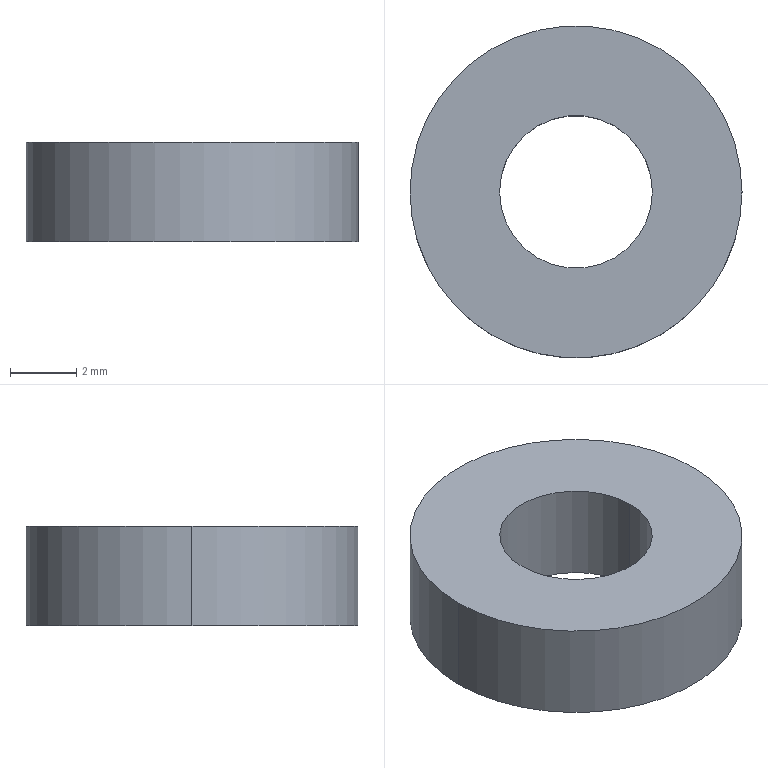Part | SolidWorks | features Extrusion 1 | 1 solid | 6 faces | box 10 x 10 x 3 mm | volume 185.762 mm3 | cylinder 4 | plane 2 | commonest cylinder face diameters 4.6 x2 10 x2
STEP:
#1=CARTESIAN_POINT('',(-2.3,0.,3.));
#2=VERTEX_POINT('',#1);
#3=CARTESIAN_POINT('',(2.3,0.,3.));
#4=VERTEX_POINT('',#3);
#5=CARTESIAN_POINT('',(0.,0.,3.));
#6=DIRECTION('',(0.,0.,1.));
#7=DIRECTION('',(1.,0.,0.));
#8=AXIS2_PLACEMENT_3D('',#5,#6,#7);
#9=CIRCLE('',#8,2.3);
#10=EDGE_CURVE('',#2,#4,#9,.T.);
#11=ORIENTED_EDGE('',*,*,#10,.T.);
#12=CARTESIAN_POINT('',(2.3,0.,0.));
#13=VERTEX_POINT('',#12);
#14=CARTESIAN_POINT('',(2.3,0.,3.));
#15=DIRECTION('',(0.,0.,-1.));
#16=VECTOR('',#15,1000.);
#17=LINE('',#14,#16);
#18=EDGE_CURVE('',#4,#13,#17,.T.);
#19=ORIENTED_EDGE('',*,*,#18,.T.);
#20=CARTESIAN_POINT('',(-2.3,0.,0.));
#21=VERTEX_POINT('',#20);
#22=CARTESIAN_POINT('',(0.,0.,0.));
#23=DIRECTION('',(0.,0.,1.));
#24=DIRECTION('',(1.,0.,0.));
#25=AXIS2_PLACEMENT_3D('',#22,#23,#24);
#26=CIRCLE('',#25,2.3);
#27=EDGE_CURVE('',#21,#13,#26,.T.);
#28=ORIENTED_EDGE('',*,*,#27,.F.);
#29=CARTESIAN_POINT('',(-2.3,0.,3.));
#30=DIRECTION('',(0.,0.,-1.));
#31=VECTOR('',#30,1000.);
#32=LINE('',#29,#31);
#33=EDGE_CURVE('',#2,#21,#32,.T.);
#34=ORIENTED_EDGE('',*,*,#33,.F.);
#35=EDGE_LOOP('',(#11,#19,#28,#34));
#36=FACE_OUTER_BOUND('',#35,.T.);
#37=CARTESIAN_POINT('',(0.,0.,3.));
#38=DIRECTION('',(0.,0.,-1.));
#39=DIRECTION('',(-1.,0.,0.));
#40=AXIS2_PLACEMENT_3D('',#37,#38,#39);
#41=CYLINDRICAL_SURFACE('',#40,2.3);
#42=ADVANCED_FACE('',(#36),#41,.F.);
#43=CARTESIAN_POINT('',(5.,0.,3.));
#44=VERTEX_POINT('',#43);
#45=CARTESIAN_POINT('',(-5.,0.,3.));
#46=VERTEX_POINT('',#45);
#47=CARTESIAN_POINT('',(0.,0.,3.));
#48=DIRECTION('',(0.,0.,1.));
#49=DIRECTION('',(1.,0.,0.));
#50=AXIS2_PLACEMENT_3D('',#47,#48,#49);
#51=CIRCLE('',#50,5.);
#52=EDGE_CURVE('',#44,#46,#51,.T.);
#53=ORIENTED_EDGE('',*,*,#52,.F.);
#54=CARTESIAN_POINT('',(5.,0.,0.));
#55=VERTEX_POINT('',#54);
#56=CARTESIAN_POINT('',(5.,0.,3.));
#57=DIRECTION('',(0.,0.,-1.));
#58=VECTOR('',#57,1000.);
#59=LINE('',#56,#58);
#60=EDGE_CURVE('',#44,#55,#59,.T.);
#61=ORIENTED_EDGE('',*,*,#60,.T.);
#62=CARTESIAN_POINT('',(-5.,0.,0.));
#63=VERTEX_POINT('',#62);
#64=CARTESIAN_POINT('',(0.,0.,0.));
#65=DIRECTION('',(0.,0.,1.));
#66=DIRECTION('',(1.,0.,0.));
#67=AXIS2_PLACEMENT_3D('',#64,#65,#66);
#68=CIRCLE('',#67,5.);
#69=EDGE_CURVE('',#55,#63,#68,.T.);
#70=ORIENTED_EDGE('',*,*,#69,.T.);
#71=CARTESIAN_POINT('',(-5.,0.,3.));
#72=DIRECTION('',(0.,0.,-1.));
#73=VECTOR('',#72,1000.);
#74=LINE('',#71,#73);
#75=EDGE_CURVE('',#46,#63,#74,.T.);
#76=ORIENTED_EDGE('',*,*,#75,.F.);
#77=EDGE_LOOP('',(#53,#61,#70,#76));
#78=FACE_OUTER_BOUND('',#77,.T.);
#79=CARTESIAN_POINT('',(0.,0.,3.));
#80=DIRECTION('',(0.,0.,-1.));
#81=DIRECTION('',(-1.,0.,0.));
#82=AXIS2_PLACEMENT_3D('',#79,#80,#81);
#83=CYLINDRICAL_SURFACE('',#82,5.);
#84=ADVANCED_FACE('',(#78),#83,.T.);
#85=CARTESIAN_POINT('',(0.,0.,3.));
#86=DIRECTION('',(0.,0.,1.));
#87=DIRECTION('',(1.,0.,0.));
#88=AXIS2_PLACEMENT_3D('',#85,#86,#87);
#89=CIRCLE('',#88,5.);
#90=EDGE_CURVE('',#46,#44,#89,.T.);
#91=ORIENTED_EDGE('',*,*,#90,.T.);
#92=ORIENTED_EDGE('',*,*,#52,.T.);
#93=EDGE_LOOP('',(#91,#92));
#94=FACE_OUTER_BOUND('',#93,.T.);
#95=ORIENTED_EDGE('',*,*,#10,.F.);
#96=CARTESIAN_POINT('',(0.,0.,3.));
#97=DIRECTION('',(0.,0.,1.));
#98=DIRECTION('',(1.,0.,0.));
#99=AXIS2_PLACEMENT_3D('',#96,#97,#98);
#100=CIRCLE('',#99,2.3);
#101=EDGE_CURVE('',#4,#2,#100,.T.);
#102=ORIENTED_EDGE('',*,*,#101,.F.);
#103=EDGE_LOOP('',(#95,#102));
#104=FACE_BOUND('',#103,.T.);
#105=CARTESIAN_POINT('',(0.,0.,3.));
#106=DIRECTION('',(0.,0.,1.));
#107=DIRECTION('',(1.,0.,0.));
#108=AXIS2_PLACEMENT_3D('',#105,#106,#107);
#109=PLANE('',#108);
#110=ADVANCED_FACE('',(#94,#104),#109,.T.);
#111=CARTESIAN_POINT('',(0.,0.,0.));
#112=DIRECTION('',(0.,0.,1.));
#113=DIRECTION('',(1.,0.,0.));
#114=AXIS2_PLACEMENT_3D('',#111,#112,#113);
#115=CIRCLE('',#114,5.);
#116=EDGE_CURVE('',#63,#55,#115,.T.);
#117=ORIENTED_EDGE('',*,*,#116,.F.);
#118=ORIENTED_EDGE('',*,*,#69,.F.);
#119=EDGE_LOOP('',(#117,#118));
#120=FACE_OUTER_BOUND('',#119,.T.);
#121=ORIENTED_EDGE('',*,*,#27,.T.);
#122=CARTESIAN_POINT('',(0.,0.,0.));
#123=DIRECTION('',(0.,0.,1.));
#124=DIRECTION('',(1.,0.,0.));
#125=AXIS2_PLACEMENT_3D('',#122,#123,#124);
#126=CIRCLE('',#125,2.3);
#127=EDGE_CURVE('',#13,#21,#126,.T.);
#128=ORIENTED_EDGE('',*,*,#127,.T.);
#129=EDGE_LOOP('',(#121,#128));
#130=FACE_BOUND('',#129,.T.);
#131=CARTESIAN_POINT('',(0.,0.,0.));
#132=DIRECTION('',(0.,0.,1.));
#133=DIRECTION('',(1.,0.,0.));
#134=AXIS2_PLACEMENT_3D('',#131,#132,#133);
#135=PLANE('',#134);
#136=ADVANCED_FACE('',(#120,#130),#135,.F.);
#137=ORIENTED_EDGE('',*,*,#60,.F.);
#138=ORIENTED_EDGE('',*,*,#90,.F.);
#139=ORIENTED_EDGE('',*,*,#75,.T.);
#140=ORIENTED_EDGE('',*,*,#116,.T.);
#141=EDGE_LOOP('',(#137,#138,#139,#140));
#142=FACE_OUTER_BOUND('',#141,.T.);
#143=CARTESIAN_POINT('',(0.,0.,3.));
#144=DIRECTION('',(0.,0.,-1.));
#145=DIRECTION('',(-1.,0.,0.));
#146=AXIS2_PLACEMENT_3D('',#143,#144,#145);
#147=CYLINDRICAL_SURFACE('',#146,5.);
#148=ADVANCED_FACE('',(#142),#147,.T.);
#149=ORIENTED_EDGE('',*,*,#18,.F.);
#150=ORIENTED_EDGE('',*,*,#101,.T.);
#151=ORIENTED_EDGE('',*,*,#33,.T.);
#152=ORIENTED_EDGE('',*,*,#127,.F.);
#153=EDGE_LOOP('',(#149,#150,#151,#152));
#154=FACE_OUTER_BOUND('',#153,.T.);
#155=CARTESIAN_POINT('',(0.,0.,3.));
#156=DIRECTION('',(0.,0.,-1.));
#157=DIRECTION('',(-1.,0.,0.));
#158=AXIS2_PLACEMENT_3D('',#155,#156,#157);
#159=CYLINDRICAL_SURFACE('',#158,2.3);
#160=ADVANCED_FACE('',(#154),#159,.F.);
#161=CLOSED_SHELL('',(#42,#84,#110,#136,#148,#160));
#162=MANIFOLD_SOLID_BREP('',#161);
#163=CARTESIAN_POINT('',(0.,0.,0.));
#164=DIRECTION('',(0.,0.,1.));
#165=DIRECTION('',(1.,0.,0.));
#166=AXIS2_PLACEMENT_3D('',#163,#164,#165);
#167=(LENGTH_UNIT()NAMED_UNIT(*)SI_UNIT(.MILLI.,.METRE.));
#168=UNCERTAINTY_MEASURE_WITH_UNIT(LENGTH_MEASURE(0.00001),#167,'','');
#169=(NAMED_UNIT(*)PLANE_ANGLE_UNIT()SI_UNIT($,.RADIAN.));
#170=(NAMED_UNIT(*)SI_UNIT($,.STERADIAN.)SOLID_ANGLE_UNIT());
#171=(GEOMETRIC_REPRESENTATION_CONTEXT(3)GLOBAL_UNCERTAINTY_ASSIGNED_CONTEXT((#168))GLOBAL_UNIT_ASSIGNED_CONTEXT((#167,#169,#170))REPRESENTATION_CONTEXT('',''));
#172=ADVANCED_BREP_SHAPE_REPRESENTATION('',(#162,#166),#171);